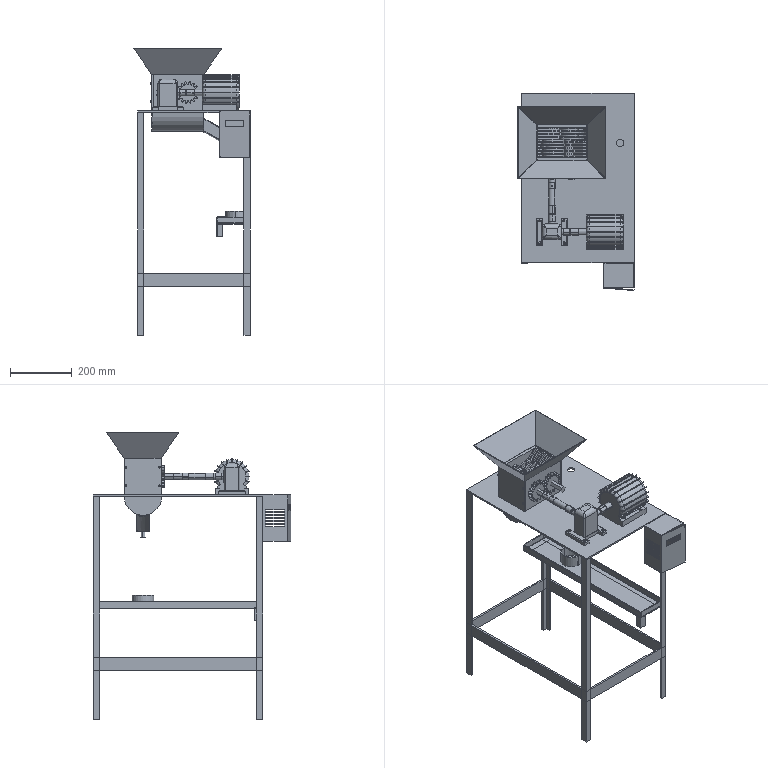Part | NX | 108 solids | 1845 faces | box 377.735 x 640.424 x 932.038 mm | volume 5983886 mm3 | plane 1045 | cylinder 683 | torus 65 | cone 48 | spline 4 | commonest cylinder face diameters 6 x110 60 x100 80 x80 25.6 x72 50 x60 3.3 x44